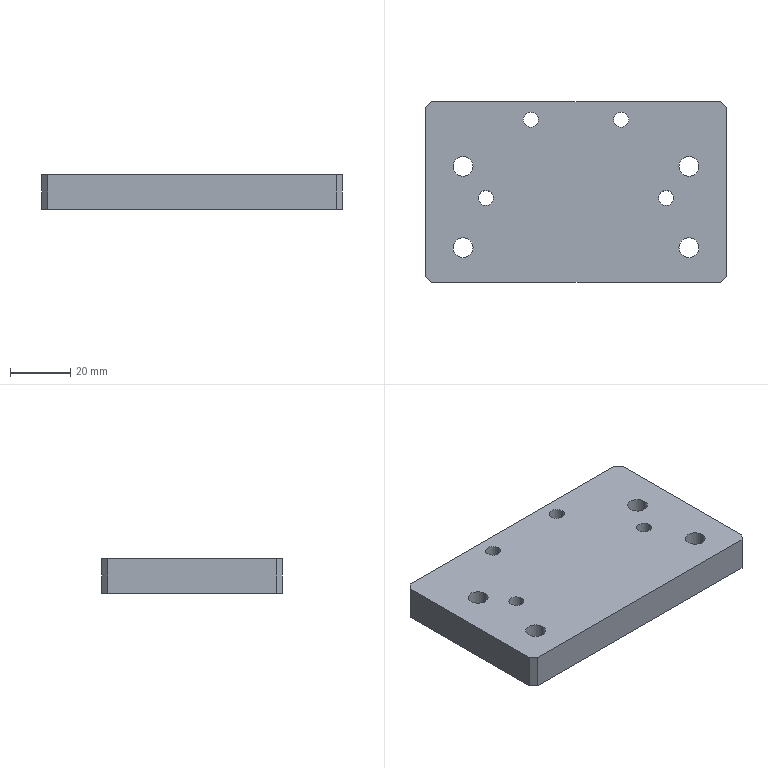Part | STEP file | FBDS-CS-003 | 1 solid | 38 faces | box 100 x 60 x 11.5 mm | volume 64777 mm3 | cylinder 24 | plane 14 | commonest cylinder face diameters 5 x8 6.6 x8 11 x8
STEP:
#1=CARTESIAN_POINT('',(17.5,24.,11.5));
#2=VERTEX_POINT('',#1);
#3=CARTESIAN_POINT('',(12.5,24.,11.5));
#4=VERTEX_POINT('',#3);
#5=CARTESIAN_POINT('',(15.,24.,11.5));
#6=DIRECTION('',(0.,0.,-1.));
#7=DIRECTION('',(-1.,0.,0.));
#8=AXIS2_PLACEMENT_3D('',#5,#6,#7);
#9=CIRCLE('',#8,2.5);
#10=EDGE_CURVE('',#2,#4,#9,.T.);
#11=ORIENTED_EDGE('',*,*,#10,.F.);
#12=CARTESIAN_POINT('',(17.5,24.,0.));
#13=VERTEX_POINT('',#12);
#14=CARTESIAN_POINT('',(17.5,24.,0.));
#15=DIRECTION('',(0.,0.,-1.));
#16=VECTOR('',#15,1000.);
#17=LINE('',#14,#16);
#18=EDGE_CURVE('',#2,#13,#17,.T.);
#19=ORIENTED_EDGE('',*,*,#18,.T.);
#20=CARTESIAN_POINT('',(12.5,24.,0.));
#21=VERTEX_POINT('',#20);
#22=CARTESIAN_POINT('',(15.,24.,0.));
#23=DIRECTION('',(0.,0.,-1.));
#24=DIRECTION('',(-1.,0.,0.));
#25=AXIS2_PLACEMENT_3D('',#22,#23,#24);
#26=CIRCLE('',#25,2.5);
#27=EDGE_CURVE('',#13,#21,#26,.T.);
#28=ORIENTED_EDGE('',*,*,#27,.T.);
#29=CARTESIAN_POINT('',(12.5,24.,0.));
#30=DIRECTION('',(0.,0.,-1.));
#31=VECTOR('',#30,1000.);
#32=LINE('',#29,#31);
#33=EDGE_CURVE('',#4,#21,#32,.T.);
#34=ORIENTED_EDGE('',*,*,#33,.F.);
#35=EDGE_LOOP('',(#11,#19,#28,#34));
#36=FACE_OUTER_BOUND('',#35,.T.);
#37=CARTESIAN_POINT('',(15.,24.,0.));
#38=DIRECTION('',(0.,0.,-1.));
#39=DIRECTION('',(-1.,0.,0.));
#40=AXIS2_PLACEMENT_3D('',#37,#38,#39);
#41=CYLINDRICAL_SURFACE('',#40,2.5);
#42=ADVANCED_FACE('',(#36),#41,.F.);
#43=CARTESIAN_POINT('',(-12.5,24.,11.5));
#44=VERTEX_POINT('',#43);
#45=CARTESIAN_POINT('',(-17.5,24.,11.5));
#46=VERTEX_POINT('',#45);
#47=CARTESIAN_POINT('',(-15.,24.,11.5));
#48=DIRECTION('',(0.,0.,-1.));
#49=DIRECTION('',(-1.,0.,0.));
#50=AXIS2_PLACEMENT_3D('',#47,#48,#49);
#51=CIRCLE('',#50,2.5);
#52=EDGE_CURVE('',#44,#46,#51,.T.);
#53=ORIENTED_EDGE('',*,*,#52,.F.);
#54=CARTESIAN_POINT('',(-12.5,24.,0.));
#55=VERTEX_POINT('',#54);
#56=CARTESIAN_POINT('',(-12.5,24.,0.));
#57=DIRECTION('',(0.,0.,-1.));
#58=VECTOR('',#57,1000.);
#59=LINE('',#56,#58);
#60=EDGE_CURVE('',#44,#55,#59,.T.);
#61=ORIENTED_EDGE('',*,*,#60,.T.);
#62=CARTESIAN_POINT('',(-17.5,24.,0.));
#63=VERTEX_POINT('',#62);
#64=CARTESIAN_POINT('',(-15.,24.,0.));
#65=DIRECTION('',(0.,0.,-1.));
#66=DIRECTION('',(-1.,0.,0.));
#67=AXIS2_PLACEMENT_3D('',#64,#65,#66);
#68=CIRCLE('',#67,2.5);
#69=EDGE_CURVE('',#55,#63,#68,.T.);
#70=ORIENTED_EDGE('',*,*,#69,.T.);
#71=CARTESIAN_POINT('',(-17.5,24.,0.));
#72=DIRECTION('',(0.,0.,-1.));
#73=VECTOR('',#72,1000.);
#74=LINE('',#71,#73);
#75=EDGE_CURVE('',#46,#63,#74,.T.);
#76=ORIENTED_EDGE('',*,*,#75,.F.);
#77=EDGE_LOOP('',(#53,#61,#70,#76));
#78=FACE_OUTER_BOUND('',#77,.T.);
#79=CARTESIAN_POINT('',(-15.,24.,0.));
#80=DIRECTION('',(0.,0.,-1.));
#81=DIRECTION('',(-1.,0.,0.));
#82=AXIS2_PLACEMENT_3D('',#79,#80,#81);
#83=CYLINDRICAL_SURFACE('',#82,2.5);
#84=ADVANCED_FACE('',(#78),#83,.F.);
#85=CARTESIAN_POINT('',(32.5,-2.,11.5));
#86=VERTEX_POINT('',#85);
#87=CARTESIAN_POINT('',(27.5,-2.,11.5));
#88=VERTEX_POINT('',#87);
#89=CARTESIAN_POINT('',(30.,-2.,11.5));
#90=DIRECTION('',(0.,0.,-1.));
#91=DIRECTION('',(-1.,0.,0.));
#92=AXIS2_PLACEMENT_3D('',#89,#90,#91);
#93=CIRCLE('',#92,2.5);
#94=EDGE_CURVE('',#86,#88,#93,.T.);
#95=ORIENTED_EDGE('',*,*,#94,.F.);
#96=CARTESIAN_POINT('',(32.5,-2.,0.));
#97=VERTEX_POINT('',#96);
#98=CARTESIAN_POINT('',(32.5,-2.,0.));
#99=DIRECTION('',(0.,0.,-1.));
#100=VECTOR('',#99,1000.);
#101=LINE('',#98,#100);
#102=EDGE_CURVE('',#86,#97,#101,.T.);
#103=ORIENTED_EDGE('',*,*,#102,.T.);
#104=CARTESIAN_POINT('',(27.5,-2.,0.));
#105=VERTEX_POINT('',#104);
#106=CARTESIAN_POINT('',(30.,-2.,0.));
#107=DIRECTION('',(0.,0.,-1.));
#108=DIRECTION('',(-1.,0.,0.));
#109=AXIS2_PLACEMENT_3D('',#106,#107,#108);
#110=CIRCLE('',#109,2.5);
#111=EDGE_CURVE('',#97,#105,#110,.T.);
#112=ORIENTED_EDGE('',*,*,#111,.T.);
#113=CARTESIAN_POINT('',(27.5,-2.,0.));
#114=DIRECTION('',(0.,0.,-1.));
#115=VECTOR('',#114,1000.);
#116=LINE('',#113,#115);
#117=EDGE_CURVE('',#88,#105,#116,.T.);
#118=ORIENTED_EDGE('',*,*,#117,.F.);
#119=EDGE_LOOP('',(#95,#103,#112,#118));
#120=FACE_OUTER_BOUND('',#119,.T.);
#121=CARTESIAN_POINT('',(30.,-2.,0.));
#122=DIRECTION('',(0.,0.,-1.));
#123=DIRECTION('',(-1.,0.,0.));
#124=AXIS2_PLACEMENT_3D('',#121,#122,#123);
#125=CYLINDRICAL_SURFACE('',#124,2.5);
#126=ADVANCED_FACE('',(#120),#125,.F.);
#127=CARTESIAN_POINT('',(-27.5,-2.,11.5));
#128=VERTEX_POINT('',#127);
#129=CARTESIAN_POINT('',(-32.5,-2.,11.5));
#130=VERTEX_POINT('',#129);
#131=CARTESIAN_POINT('',(-30.,-2.,11.5));
#132=DIRECTION('',(0.,0.,-1.));
#133=DIRECTION('',(-1.,0.,0.));
#134=AXIS2_PLACEMENT_3D('',#131,#132,#133);
#135=CIRCLE('',#134,2.5);
#136=EDGE_CURVE('',#128,#130,#135,.T.);
#137=ORIENTED_EDGE('',*,*,#136,.F.);
#138=CARTESIAN_POINT('',(-27.5,-2.,0.));
#139=VERTEX_POINT('',#138);
#140=CARTESIAN_POINT('',(-27.5,-2.,0.));
#141=DIRECTION('',(0.,0.,-1.));
#142=VECTOR('',#141,1000.);
#143=LINE('',#140,#142);
#144=EDGE_CURVE('',#128,#139,#143,.T.);
#145=ORIENTED_EDGE('',*,*,#144,.T.);
#146=CARTESIAN_POINT('',(-32.5,-2.,0.));
#147=VERTEX_POINT('',#146);
#148=CARTESIAN_POINT('',(-30.,-2.,0.));
#149=DIRECTION('',(0.,0.,-1.));
#150=DIRECTION('',(-1.,0.,0.));
#151=AXIS2_PLACEMENT_3D('',#148,#149,#150);
#152=CIRCLE('',#151,2.5);
#153=EDGE_CURVE('',#139,#147,#152,.T.);
#154=ORIENTED_EDGE('',*,*,#153,.T.);
#155=CARTESIAN_POINT('',(-32.5,-2.,0.));
#156=DIRECTION('',(0.,0.,-1.));
#157=VECTOR('',#156,1000.);
#158=LINE('',#155,#157);
#159=EDGE_CURVE('',#130,#147,#158,.T.);
#160=ORIENTED_EDGE('',*,*,#159,.F.);
#161=EDGE_LOOP('',(#137,#145,#154,#160));
#162=FACE_OUTER_BOUND('',#161,.T.);
#163=CARTESIAN_POINT('',(-30.,-2.,0.));
#164=DIRECTION('',(0.,0.,-1.));
#165=DIRECTION('',(-1.,0.,0.));
#166=AXIS2_PLACEMENT_3D('',#163,#164,#165);
#167=CYLINDRICAL_SURFACE('',#166,2.5);
#168=ADVANCED_FACE('',(#162),#167,.F.);
#169=CARTESIAN_POINT('',(43.,8.5,6.8));
#170=VERTEX_POINT('',#169);
#171=CARTESIAN_POINT('',(32.,8.5,6.8));
#172=VERTEX_POINT('',#171);
#173=CARTESIAN_POINT('',(37.5,8.5,6.8));
#174=DIRECTION('',(0.,0.,-1.));
#175=DIRECTION('',(-1.,0.,0.));
#176=AXIS2_PLACEMENT_3D('',#173,#174,#175);
#177=CIRCLE('',#176,5.5);
#178=EDGE_CURVE('',#170,#172,#177,.T.);
#179=ORIENTED_EDGE('',*,*,#178,.F.);
#180=CARTESIAN_POINT('',(43.,8.5,0.));
#181=VERTEX_POINT('',#180);
#182=CARTESIAN_POINT('',(43.,8.5,0.));
#183=DIRECTION('',(0.,0.,-1.));
#184=VECTOR('',#183,1000.);
#185=LINE('',#182,#184);
#186=EDGE_CURVE('',#170,#181,#185,.T.);
#187=ORIENTED_EDGE('',*,*,#186,.T.);
#188=CARTESIAN_POINT('',(32.,8.5,0.));
#189=VERTEX_POINT('',#188);
#190=CARTESIAN_POINT('',(37.5,8.5,0.));
#191=DIRECTION('',(0.,0.,-1.));
#192=DIRECTION('',(-1.,0.,0.));
#193=AXIS2_PLACEMENT_3D('',#190,#191,#192);
#194=CIRCLE('',#193,5.5);
#195=EDGE_CURVE('',#181,#189,#194,.T.);
#196=ORIENTED_EDGE('',*,*,#195,.T.);
#197=CARTESIAN_POINT('',(32.,8.5,0.));
#198=DIRECTION('',(0.,0.,-1.));
#199=VECTOR('',#198,1000.);
#200=LINE('',#197,#199);
#201=EDGE_CURVE('',#172,#189,#200,.T.);
#202=ORIENTED_EDGE('',*,*,#201,.F.);
#203=EDGE_LOOP('',(#179,#187,#196,#202));
#204=FACE_OUTER_BOUND('',#203,.T.);
#205=CARTESIAN_POINT('',(37.5,8.5,0.));
#206=DIRECTION('',(0.,0.,-1.));
#207=DIRECTION('',(-1.,0.,0.));
#208=AXIS2_PLACEMENT_3D('',#205,#206,#207);
#209=CYLINDRICAL_SURFACE('',#208,5.5);
#210=ADVANCED_FACE('',(#204),#209,.F.);
#211=CARTESIAN_POINT('',(40.8,8.5,11.5));
#212=VERTEX_POINT('',#211);
#213=CARTESIAN_POINT('',(34.2,8.5,11.5));
#214=VERTEX_POINT('',#213);
#215=CARTESIAN_POINT('',(37.5,8.5,11.5));
#216=DIRECTION('',(0.,0.,-1.));
#217=DIRECTION('',(-1.,0.,0.));
#218=AXIS2_PLACEMENT_3D('',#215,#216,#217);
#219=CIRCLE('',#218,3.3);
#220=EDGE_CURVE('',#212,#214,#219,.T.);
#221=ORIENTED_EDGE('',*,*,#220,.F.);
#222=CARTESIAN_POINT('',(40.8,8.5,6.8));
#223=VERTEX_POINT('',#222);
#224=CARTESIAN_POINT('',(40.8,8.5,0.));
#225=DIRECTION('',(0.,0.,-1.));
#226=VECTOR('',#225,1000.);
#227=LINE('',#224,#226);
#228=EDGE_CURVE('',#212,#223,#227,.T.);
#229=ORIENTED_EDGE('',*,*,#228,.T.);
#230=CARTESIAN_POINT('',(34.2,8.5,6.8));
#231=VERTEX_POINT('',#230);
#232=CARTESIAN_POINT('',(37.5,8.5,6.8));
#233=DIRECTION('',(0.,0.,-1.));
#234=DIRECTION('',(-1.,0.,0.));
#235=AXIS2_PLACEMENT_3D('',#232,#233,#234);
#236=CIRCLE('',#235,3.3);
#237=EDGE_CURVE('',#223,#231,#236,.T.);
#238=ORIENTED_EDGE('',*,*,#237,.T.);
#239=CARTESIAN_POINT('',(34.2,8.5,0.));
#240=DIRECTION('',(0.,0.,-1.));
#241=VECTOR('',#240,1000.);
#242=LINE('',#239,#241);
#243=EDGE_CURVE('',#214,#231,#242,.T.);
#244=ORIENTED_EDGE('',*,*,#243,.F.);
#245=EDGE_LOOP('',(#221,#229,#238,#244));
#246=FACE_OUTER_BOUND('',#245,.T.);
#247=CARTESIAN_POINT('',(37.5,8.5,0.));
#248=DIRECTION('',(0.,0.,-1.));
#249=DIRECTION('',(-1.,0.,0.));
#250=AXIS2_PLACEMENT_3D('',#247,#248,#249);
#251=CYLINDRICAL_SURFACE('',#250,3.3);
#252=ADVANCED_FACE('',(#246),#251,.F.);
#253=CARTESIAN_POINT('',(-32.,8.5,6.8));
#254=VERTEX_POINT('',#253);
#255=CARTESIAN_POINT('',(-43.,8.5,6.8));
#256=VERTEX_POINT('',#255);
#257=CARTESIAN_POINT('',(-37.5,8.5,6.8));
#258=DIRECTION('',(0.,0.,-1.));
#259=DIRECTION('',(-1.,0.,0.));
#260=AXIS2_PLACEMENT_3D('',#257,#258,#259);
#261=CIRCLE('',#260,5.5);
#262=EDGE_CURVE('',#254,#256,#261,.T.);
#263=ORIENTED_EDGE('',*,*,#262,.F.);
#264=CARTESIAN_POINT('',(-32.,8.5,0.));
#265=VERTEX_POINT('',#264);
#266=CARTESIAN_POINT('',(-32.,8.5,0.));
#267=DIRECTION('',(0.,0.,-1.));
#268=VECTOR('',#267,1000.);
#269=LINE('',#266,#268);
#270=EDGE_CURVE('',#254,#265,#269,.T.);
#271=ORIENTED_EDGE('',*,*,#270,.T.);
#272=CARTESIAN_POINT('',(-43.,8.5,0.));
#273=VERTEX_POINT('',#272);
#274=CARTESIAN_POINT('',(-37.5,8.5,0.));
#275=DIRECTION('',(0.,0.,-1.));
#276=DIRECTION('',(-1.,0.,0.));
#277=AXIS2_PLACEMENT_3D('',#274,#275,#276);
#278=CIRCLE('',#277,5.5);
#279=EDGE_CURVE('',#265,#273,#278,.T.);
#280=ORIENTED_EDGE('',*,*,#279,.T.);
#281=CARTESIAN_POINT('',(-43.,8.5,0.));
#282=DIRECTION('',(0.,0.,-1.));
#283=VECTOR('',#282,1000.);
#284=LINE('',#281,#283);
#285=EDGE_CURVE('',#256,#273,#284,.T.);
#286=ORIENTED_EDGE('',*,*,#285,.F.);
#287=EDGE_LOOP('',(#263,#271,#280,#286));
#288=FACE_OUTER_BOUND('',#287,.T.);
#289=CARTESIAN_POINT('',(-37.5,8.5,0.));
#290=DIRECTION('',(0.,0.,-1.));
#291=DIRECTION('',(-1.,0.,0.));
#292=AXIS2_PLACEMENT_3D('',#289,#290,#291);
#293=CYLINDRICAL_SURFACE('',#292,5.5);
#294=ADVANCED_FACE('',(#288),#293,.F.);
#295=CARTESIAN_POINT('',(-34.2,8.5,11.5));
#296=VERTEX_POINT('',#295);
#297=CARTESIAN_POINT('',(-40.8,8.5,11.5));
#298=VERTEX_POINT('',#297);
#299=CARTESIAN_POINT('',(-37.5,8.5,11.5));
#300=DIRECTION('',(0.,0.,-1.));
#301=DIRECTION('',(-1.,0.,0.));
#302=AXIS2_PLACEMENT_3D('',#299,#300,#301);
#303=CIRCLE('',#302,3.3);
#304=EDGE_CURVE('',#296,#298,#303,.T.);
#305=ORIENTED_EDGE('',*,*,#304,.F.);
#306=CARTESIAN_POINT('',(-34.2,8.5,6.8));
#307=VERTEX_POINT('',#306);
#308=CARTESIAN_POINT('',(-34.2,8.5,0.));
#309=DIRECTION('',(0.,0.,-1.));
#310=VECTOR('',#309,1000.);
#311=LINE('',#308,#310);
#312=EDGE_CURVE('',#296,#307,#311,.T.);
#313=ORIENTED_EDGE('',*,*,#312,.T.);
#314=CARTESIAN_POINT('',(-40.8,8.5,6.8));
#315=VERTEX_POINT('',#314);
#316=CARTESIAN_POINT('',(-37.5,8.5,6.8));
#317=DIRECTION('',(0.,0.,-1.));
#318=DIRECTION('',(-1.,0.,0.));
#319=AXIS2_PLACEMENT_3D('',#316,#317,#318);
#320=CIRCLE('',#319,3.3);
#321=EDGE_CURVE('',#307,#315,#320,.T.);
#322=ORIENTED_EDGE('',*,*,#321,.T.);
#323=CARTESIAN_POINT('',(-40.8,8.5,0.));
#324=DIRECTION('',(0.,0.,-1.));
#325=VECTOR('',#324,1000.);
#326=LINE('',#323,#325);
#327=EDGE_CURVE('',#298,#315,#326,.T.);
#328=ORIENTED_EDGE('',*,*,#327,.F.);
#329=EDGE_LOOP('',(#305,#313,#322,#328));
#330=FACE_OUTER_BOUND('',#329,.T.);
#331=CARTESIAN_POINT('',(-37.5,8.5,0.));
#332=DIRECTION('',(0.,0.,-1.));
#333=DIRECTION('',(-1.,0.,0.));
#334=AXIS2_PLACEMENT_3D('',#331,#332,#333);
#335=CYLINDRICAL_SURFACE('',#334,3.3);
#336=ADVANCED_FACE('',(#330),#335,.F.);
#337=CARTESIAN_POINT('',(-32.,-18.5,6.8));
#338=VERTEX_POINT('',#337);
#339=CARTESIAN_POINT('',(-43.,-18.5,6.8));
#340=VERTEX_POINT('',#339);
#341=CARTESIAN_POINT('',(-37.5,-18.5,6.8));
#342=DIRECTION('',(0.,0.,-1.));
#343=DIRECTION('',(-1.,0.,0.));
#344=AXIS2_PLACEMENT_3D('',#341,#342,#343);
#345=CIRCLE('',#344,5.5);
#346=EDGE_CURVE('',#338,#340,#345,.T.);
#347=ORIENTED_EDGE('',*,*,#346,.F.);
#348=CARTESIAN_POINT('',(-32.,-18.5,0.));
#349=VERTEX_POINT('',#348);
#350=CARTESIAN_POINT('',(-32.,-18.5,0.));
#351=DIRECTION('',(0.,0.,-1.));
#352=VECTOR('',#351,1000.);
#353=LINE('',#350,#352);
#354=EDGE_CURVE('',#338,#349,#353,.T.);
#355=ORIENTED_EDGE('',*,*,#354,.T.);
#356=CARTESIAN_POINT('',(-43.,-18.5,0.));
#357=VERTEX_POINT('',#356);
#358=CARTESIAN_POINT('',(-37.5,-18.5,0.));
#359=DIRECTION('',(0.,0.,-1.));
#360=DIRECTION('',(-1.,0.,0.));
#361=AXIS2_PLACEMENT_3D('',#358,#359,#360);
#362=CIRCLE('',#361,5.5);
#363=EDGE_CURVE('',#349,#357,#362,.T.);
#364=ORIENTED_EDGE('',*,*,#363,.T.);
#365=CARTESIAN_POINT('',(-43.,-18.5,0.));
#366=DIRECTION('',(0.,0.,-1.));
#367=VECTOR('',#366,1000.);
#368=LINE('',#365,#367);
#369=EDGE_CURVE('',#340,#357,#368,.T.);
#370=ORIENTED_EDGE('',*,*,#369,.F.);
#371=EDGE_LOOP('',(#347,#355,#364,#370));
#372=FACE_OUTER_BOUND('',#371,.T.);
#373=CARTESIAN_POINT('',(-37.5,-18.5,0.));
#374=DIRECTION('',(0.,0.,-1.));
#375=DIRECTION('',(-1.,0.,0.));
#376=AXIS2_PLACEMENT_3D('',#373,#374,#375);
#377=CYLINDRICAL_SURFACE('',#376,5.5);
#378=ADVANCED_FACE('',(#372),#377,.F.);
#379=CARTESIAN_POINT('',(-34.2,-18.5,11.5));
#380=VERTEX_POINT('',#379);
#381=CARTESIAN_POINT('',(-40.8,-18.5,11.5));
#382=VERTEX_POINT('',#381);
#383=CARTESIAN_POINT('',(-37.5,-18.5,11.5));
#384=DIRECTION('',(0.,0.,-1.));
#385=DIRECTION('',(-1.,0.,0.));
#386=AXIS2_PLACEMENT_3D('',#383,#384,#385);
#387=CIRCLE('',#386,3.3);
#388=EDGE_CURVE('',#380,#382,#387,.T.);
#389=ORIENTED_EDGE('',*,*,#388,.F.);
#390=CARTESIAN_POINT('',(-34.2,-18.5,6.8));
#391=VERTEX_POINT('',#390);
#392=CARTESIAN_POINT('',(-34.2,-18.5,0.));
#393=DIRECTION('',(0.,0.,-1.));
#394=VECTOR('',#393,1000.);
#395=LINE('',#392,#394);
#396=EDGE_CURVE('',#380,#391,#395,.T.);
#397=ORIENTED_EDGE('',*,*,#396,.T.);
#398=CARTESIAN_POINT('',(-40.8,-18.5,6.8));
#399=VERTEX_POINT('',#398);
#400=CARTESIAN_POINT('',(-37.5,-18.5,6.8));
#401=DIRECTION('',(0.,0.,-1.));
#402=DIRECTION('',(-1.,0.,0.));
#403=AXIS2_PLACEMENT_3D('',#400,#401,#402);
#404=CIRCLE('',#403,3.3);
#405=EDGE_CURVE('',#391,#399,#404,.T.);
#406=ORIENTED_EDGE('',*,*,#405,.T.);
#407=CARTESIAN_POINT('',(-40.8,-18.5,0.));
#408=DIRECTION('',(0.,0.,-1.));
#409=VECTOR('',#408,1000.);
#410=LINE('',#407,#409);
#411=EDGE_CURVE('',#382,#399,#410,.T.);
#412=ORIENTED_EDGE('',*,*,#411,.F.);
#413=EDGE_LOOP('',(#389,#397,#406,#412));
#414=FACE_OUTER_BOUND('',#413,.T.);
#415=CARTESIAN_POINT('',(-37.5,-18.5,0.));
#416=DIRECTION('',(0.,0.,-1.));
#417=DIRECTION('',(-1.,0.,0.));
#418=AXIS2_PLACEMENT_3D('',#415,#416,#417);
#419=CYLINDRICAL_SURFACE('',#418,3.3);
#420=ADVANCED_FACE('',(#414),#419,.F.);
#421=CARTESIAN_POINT('',(43.,-18.5,6.8));
#422=VERTEX_POINT('',#421);
#423=CARTESIAN_POINT('',(32.,-18.5,6.8));
#424=VERTEX_POINT('',#423);
#425=CARTESIAN_POINT('',(37.5,-18.5,6.8));
#426=DIRECTION('',(0.,0.,-1.));
#427=DIRECTION('',(-1.,0.,0.));
#428=AXIS2_PLACEMENT_3D('',#425,#426,#427);
#429=CIRCLE('',#428,5.5);
#430=EDGE_CURVE('',#422,#424,#429,.T.);
#431=ORIENTED_EDGE('',*,*,#430,.F.);
#432=CARTESIAN_POINT('',(43.,-18.5,0.));
#433=VERTEX_POINT('',#432);
#434=CARTESIAN_POINT('',(43.,-18.5,0.));
#435=DIRECTION('',(0.,0.,-1.));
#436=VECTOR('',#435,1000.);
#437=LINE('',#434,#436);
#438=EDGE_CURVE('',#422,#433,#437,.T.);
#439=ORIENTED_EDGE('',*,*,#438,.T.);
#440=CARTESIAN_POINT('',(32.,-18.5,0.));
#441=VERTEX_POINT('',#440);
#442=CARTESIAN_POINT('',(37.5,-18.5,0.));
#443=DIRECTION('',(0.,0.,-1.));
#444=DIRECTION('',(-1.,0.,0.));
#445=AXIS2_PLACEMENT_3D('',#442,#443,#444);
#446=CIRCLE('',#445,5.5);
#447=EDGE_CURVE('',#433,#441,#446,.T.);
#448=ORIENTED_EDGE('',*,*,#447,.T.);
#449=CARTESIAN_POINT('',(32.,-18.5,0.));
#450=DIRECTION('',(0.,0.,-1.));
#451=VECTOR('',#450,1000.);
#452=LINE('',#449,#451);
#453=EDGE_CURVE('',#424,#441,#452,.T.);
#454=ORIENTED_EDGE('',*,*,#453,.F.);
#455=EDGE_LOOP('',(#431,#439,#448,#454));
#456=FACE_OUTER_BOUND('',#455,.T.);
#457=CARTESIAN_POINT('',(37.5,-18.5,0.));
#458=DIRECTION('',(0.,0.,-1.));
#459=DIRECTION('',(-1.,0.,0.));
#460=AXIS2_PLACEMENT_3D('',#457,#458,#459);
#461=CYLINDRICAL_SURFACE('',#460,5.5);
#462=ADVANCED_FACE('',(#456),#461,.F.);
#463=CARTESIAN_POINT('',(40.8,-18.5,11.5));
#464=VERTEX_POINT('',#463);
#465=CARTESIAN_POINT('',(34.2,-18.5,11.5));
#466=VERTEX_POINT('',#465);
#467=CARTESIAN_POINT('',(37.5,-18.5,11.5));
#468=DIRECTION('',(0.,0.,-1.));
#469=DIRECTION('',(-1.,0.,0.));
#470=AXIS2_PLACEMENT_3D('',#467,#468,#469);
#471=CIRCLE('',#470,3.3);
#472=EDGE_CURVE('',#464,#466,#471,.T.);
#473=ORIENTED_EDGE('',*,*,#472,.F.);
#474=CARTESIAN_POINT('',(40.8,-18.5,6.8));
#475=VERTEX_POINT('',#474);
#476=CARTESIAN_POINT('',(40.8,-18.5,0.));
#477=DIRECTION('',(0.,0.,-1.));
#478=VECTOR('',#477,1000.);
#479=LINE('',#476,#478);
#480=EDGE_CURVE('',#464,#475,#479,.T.);
#481=ORIENTED_EDGE('',*,*,#480,.T.);
#482=CARTESIAN_POINT('',(34.2,-18.5,6.8));
#483=VERTEX_POINT('',#482);
#484=CARTESIAN_POINT('',(37.5,-18.5,6.8));
#485=DIRECTION('',(0.,0.,-1.));
#486=DIRECTION('',(-1.,0.,0.));
#487=AXIS2_PLACEMENT_3D('',#484,#485,#486);
#488=CIRCLE('',#487,3.3);
#489=EDGE_CURVE('',#475,#483,#488,.T.);
#490=ORIENTED_EDGE('',*,*,#489,.T.);
#491=CARTESIAN_POINT('',(34.2,-18.5,0.));
#492=DIRECTION('',(0.,0.,-1.));
#493=VECTOR('',#492,1000.);
#494=LINE('',#491,#493);
#495=EDGE_CURVE('',#466,#483,#494,.T.);
#496=ORIENTED_EDGE('',*,*,#495,.F.);
#497=EDGE_LOOP('',(#473,#481,#490,#496));
#498=FACE_OUTER_BOUND('',#497,.T.);
#499=CARTESIAN_POINT('',(37.5,-18.5,0.));
#500=DIRECTION('',(0.,0.,-1.));
#501=DIRECTION('',(-1.,0.,0.));
#502=AXIS2_PLACEMENT_3D('',#499,#500,#501);
#503=CYLINDRICAL_SURFACE('',#502,3.3);
#504=ADVANCED_FACE('',(#498),#503,.F.);
#505=CARTESIAN_POINT('',(50.,-28.,11.5));
#506=VERTEX_POINT('',#505);
#507=CARTESIAN_POINT('',(50.,28.,11.5));
#508=VERTEX_POINT('',#507);
#509=CARTESIAN_POINT('',(50.,-30.,11.5));
#510=DIRECTION('',(0.,1.,0.));
#511=VECTOR('',#510,1000.);
#512=LINE('',#509,#511);
#513=EDGE_CURVE('',#506,#508,#512,.T.);
#514=ORIENTED_EDGE('',*,*,#513,.F.);
#515=CARTESIAN_POINT('',(50.,-28.,0.));
#516=VERTEX_POINT('',#515);
#517=CARTESIAN_POINT('',(50.,-28.,11.5));
#518=DIRECTION('',(0.,0.,-1.));
#519=VECTOR('',#518,1000.);
#520=LINE('',#517,#519);
#521=EDGE_CURVE('',#506,#516,#520,.T.);
#522=ORIENTED_EDGE('',*,*,#521,.T.);
#523=CARTESIAN_POINT('',(50.,28.,0.));
#524=VERTEX_POINT('',#523);
#525=CARTESIAN_POINT('',(50.,-30.,0.));
#526=DIRECTION('',(0.,1.,0.));
#527=VECTOR('',#526,1000.);
#528=LINE('',#525,#527);
#529=EDGE_CURVE('',#516,#524,#528,.T.);
#530=ORIENTED_EDGE('',*,*,#529,.T.);
#531=CARTESIAN_POINT('',(50.,28.,11.5));
#532=DIRECTION('',(0.,0.,1.));
#533=VECTOR('',#532,1000.);
#534=LINE('',#531,#533);
#535=EDGE_CURVE('',#524,#508,#534,.T.);
#536=ORIENTED_EDGE('',*,*,#535,.T.);
#537=EDGE_LOOP('',(#514,#522,#530,#536));
#538=FACE_OUTER_BOUND('',#537,.T.);
#539=CARTESIAN_POINT('',(50.,-30.,11.5));
#540=DIRECTION('',(-1.,0.,0.));
#541=DIRECTION('',(0.,0.,1.));
#542=AXIS2_PLACEMENT_3D('',#539,#540,#541);
#543=PLANE('',#542);
#544=ADVANCED_FACE('',(#538),#543,.F.);
#545=CARTESIAN_POINT('',(48.,30.,0.));
#546=VERTEX_POINT('',#545);
#547=CARTESIAN_POINT('',(-48.,30.,0.));
#548=VERTEX_POINT('',#547);
#549=CARTESIAN_POINT('',(-50.,30.,0.));
#550=DIRECTION('',(-1.,0.,0.));
#551=VECTOR('',#550,1000.);
#552=LINE('',#549,#551);
#553=EDGE_CURVE('',#546,#548,#552,.T.);
#554=ORIENTED_EDGE('',*,*,#553,.T.);
#555=CARTESIAN_POINT('',(-48.,30.,11.5));
#556=VERTEX_POINT('',#555);
#557=CARTESIAN_POINT('',(-48.,30.,11.5));
#558=DIRECTION('',(0.,0.,1.));
#559=VECTOR('',#558,1000.);
#560=LINE('',#557,#559);
#561=EDGE_CURVE('',#548,#556,#560,.T.);
#562=ORIENTED_EDGE('',*,*,#561,.T.);
#563=CARTESIAN_POINT('',(48.,30.,11.5));
#564=VERTEX_POINT('',#563);
#565=CARTESIAN_POINT('',(-50.,30.,11.5));
#566=DIRECTION('',(-1.,0.,0.));
#567=VECTOR('',#566,1000.);
#568=LINE('',#565,#567);
#569=EDGE_CURVE('',#564,#556,#568,.T.);
#570=ORIENTED_EDGE('',*,*,#569,.F.);
#571=CARTESIAN_POINT('',(48.,30.,11.5));
#572=DIRECTION('',(0.,0.,-1.));
#573=VECTOR('',#572,1000.);
#574=LINE('',#571,#573);
#575=EDGE_CURVE('',#564,#546,#574,.T.);
#576=ORIENTED_EDGE('',*,*,#575,.T.);
#577=EDGE_LOOP('',(#554,#562,#570,#576));
#578=FACE_OUTER_BOUND('',#577,.T.);
#579=CARTESIAN_POINT('',(-50.,30.,11.5));
#580=DIRECTION('',(0.,-1.,0.));
#581=DIRECTION('',(0.,0.,-1.));
#582=AXIS2_PLACEMENT_3D('',#579,#580,#581);
#583=PLANE('',#582);
#584=ADVANCED_FACE('',(#578),#583,.F.);
#585=CARTESIAN_POINT('',(-50.,28.,0.));
#586=VERTEX_POINT('',#585);
#587=CARTESIAN_POINT('',(-50.,-28.,0.));
#588=VERTEX_POINT('',#587);
#589=CARTESIAN_POINT('',(-50.,-30.,0.));
#590=DIRECTION('',(0.,-1.,0.));
#591=VECTOR('',#590,1000.);
#592=LINE('',#589,#591);
#593=EDGE_CURVE('',#586,#588,#592,.T.);
#594=ORIENTED_EDGE('',*,*,#593,.T.);
#595=CARTESIAN_POINT('',(-50.,-28.,11.5));
#596=VERTEX_POINT('',#595);
#597=CARTESIAN_POINT('',(-50.,-28.,11.5));
#598=DIRECTION('',(0.,0.,1.));
#599=VECTOR('',#598,1000.);
#600=LINE('',#597,#599);
#601=EDGE_CURVE('',#588,#596,#600,.T.);
#602=ORIENTED_EDGE('',*,*,#601,.T.);
#603=CARTESIAN_POINT('',(-50.,28.,11.5));
#604=VERTEX_POINT('',#603);
#605=CARTESIAN_POINT('',(-50.,-30.,11.5));
#606=DIRECTION('',(0.,-1.,0.));
#607=VECTOR('',#606,1000.);
#608=LINE('',#605,#607);
#609=EDGE_CURVE('',#604,#596,#608,.T.);
#610=ORIENTED_EDGE('',*,*,#609,.F.);
#611=CARTESIAN_POINT('',(-50.,28.,11.5));
#612=DIRECTION('',(0.,0.,-1.));
#613=VECTOR('',#612,1000.);
#614=LINE('',#611,#613);
#615=EDGE_CURVE('',#604,#586,#614,.T.);
#616=ORIENTED_EDGE('',*,*,#615,.T.);
#617=EDGE_LOOP('',(#594,#602,#610,#616));
#618=FACE_OUTER_BOUND('',#617,.T.);
#619=CARTESIAN_POINT('',(-50.,-30.,11.5));
#620=DIRECTION('',(1.,0.,0.));
#621=DIRECTION('',(0.,0.,-1.));
#622=AXIS2_PLACEMENT_3D('',#619,#620,#621);
#623=PLANE('',#622);
#624=ADVANCED_FACE('',(#618),#623,.F.);
#625=CARTESIAN_POINT('',(-48.,-30.,11.5));
#626=VERTEX_POINT('',#625);
#627=CARTESIAN_POINT('',(48.,-30.,11.5));
#628=VERTEX_POINT('',#627);
#629=CARTESIAN_POINT('',(-50.,-30.,11.5));
#630=DIRECTION('',(1.,0.,0.));
#631=VECTOR('',#630,1000.);
#632=LINE('',#629,#631);
#633=EDGE_CURVE('',#626,#628,#632,.T.);
#634=ORIENTED_EDGE('',*,*,#633,.F.);
#635=CARTESIAN_POINT('',(-48.,-30.,0.));
#636=VERTEX_POINT('',#635);
#637=CARTESIAN_POINT('',(-48.,-30.,11.5));
#638=DIRECTION('',(0.,0.,-1.));
#639=VECTOR('',#638,1000.);
#640=LINE('',#637,#639);
#641=EDGE_CURVE('',#626,#636,#640,.T.);
#642=ORIENTED_EDGE('',*,*,#641,.T.);
#643=CARTESIAN_POINT('',(48.,-30.,0.));
#644=VERTEX_POINT('',#643);
#645=CARTESIAN_POINT('',(-50.,-30.,0.));
#646=DIRECTION('',(1.,0.,0.));
#647=VECTOR('',#646,1000.);
#648=LINE('',#645,#647);
#649=EDGE_CURVE('',#636,#644,#648,.T.);
#650=ORIENTED_EDGE('',*,*,#649,.T.);
#651=CARTESIAN_POINT('',(48.,-30.,11.5));
#652=DIRECTION('',(0.,0.,1.));
#653=VECTOR('',#652,1000.);
#654=LINE('',#651,#653);
#655=EDGE_CURVE('',#644,#628,#654,.T.);
#656=ORIENTED_EDGE('',*,*,#655,.T.);
#657=EDGE_LOOP('',(#634,#642,#650,#656));
#658=FACE_OUTER_BOUND('',#657,.T.);
#659=CARTESIAN_POINT('',(-50.,-30.,11.5));
#660=DIRECTION('',(0.,1.,0.));
#661=DIRECTION('',(0.,0.,1.));
#662=AXIS2_PLACEMENT_3D('',#659,#660,#661);
#663=PLANE('',#662);
#664=ADVANCED_FACE('',(#658),#663,.F.);
#665=CARTESIAN_POINT('',(15.,24.,11.5));
#666=DIRECTION('',(0.,0.,-1.));
#667=DIRECTION('',(-1.,0.,0.));
#668=AXIS2_PLACEMENT_3D('',#665,#666,#667);
#669=CIRCLE('',#668,2.5);
#670=EDGE_CURVE('',#4,#2,#669,.T.);
#671=ORIENTED_EDGE('',*,*,#670,.T.);
#672=ORIENTED_EDGE('',*,*,#10,.T.);
#673=EDGE_LOOP('',(#671,#672));
#674=FACE_BOUND('',#673,.T.);
#675=CARTESIAN_POINT('',(-15.,24.,11.5));
#676=DIRECTION('',(0.,0.,-1.));
#677=DIRECTION('',(-1.,0.,0.));
#678=AXIS2_PLACEMENT_3D('',#675,#676,#677);
#679=CIRCLE('',#678,2.5);
#680=EDGE_CURVE('',#46,#44,#679,.T.);
#681=ORIENTED_EDGE('',*,*,#680,.T.);
#682=ORIENTED_EDGE('',*,*,#52,.T.);
#683=EDGE_LOOP('',(#681,#682));
#684=FACE_BOUND('',#683,.T.);
#685=CARTESIAN_POINT('',(30.,-2.,11.5));
#686=DIRECTION('',(0.,0.,-1.));
#687=DIRECTION('',(-1.,0.,0.));
#688=AXIS2_PLACEMENT_3D('',#685,#686,#687);
#689=CIRCLE('',#688,2.5);
#690=EDGE_CURVE('',#88,#86,#689,.T.);
#691=ORIENTED_EDGE('',*,*,#690,.T.);
#692=ORIENTED_EDGE('',*,*,#94,.T.);
#693=EDGE_LOOP('',(#691,#692));
#694=FACE_BOUND('',#693,.T.);
#695=CARTESIAN_POINT('',(-30.,-2.,11.5));
#696=DIRECTION('',(0.,0.,-1.));
#697=DIRECTION('',(-1.,0.,0.));
#698=AXIS2_PLACEMENT_3D('',#695,#696,#697);
#699=CIRCLE('',#698,2.5);
#700=EDGE_CURVE('',#130,#128,#699,.T.);
#701=ORIENTED_EDGE('',*,*,#700,.T.);
#702=ORIENTED_EDGE('',*,*,#136,.T.);
#703=EDGE_LOOP('',(#701,#702));
#704=FACE_BOUND('',#703,.T.);
#705=CARTESIAN_POINT('',(37.5,8.5,11.5));
#706=DIRECTION('',(0.,0.,-1.));
#707=DIRECTION('',(-1.,0.,0.));
#708=AXIS2_PLACEMENT_3D('',#705,#706,#707);
#709=CIRCLE('',#708,3.3);
#710=EDGE_CURVE('',#214,#212,#709,.T.);
#711=ORIENTED_EDGE('',*,*,#710,.T.);
#712=ORIENTED_EDGE('',*,*,#220,.T.);
#713=EDGE_LOOP('',(#711,#712));
#714=FACE_BOUND('',#713,.T.);
#715=CARTESIAN_POINT('',(-37.5,8.5,11.5));
#716=DIRECTION('',(0.,0.,-1.));
#717=DIRECTION('',(-1.,0.,0.));
#718=AXIS2_PLACEMENT_3D('',#715,#716,#717);
#719=CIRCLE('',#718,3.3);
#720=EDGE_CURVE('',#298,#296,#719,.T.);
#721=ORIENTED_EDGE('',*,*,#720,.T.);
#722=ORIENTED_EDGE('',*,*,#304,.T.);
#723=EDGE_LOOP('',(#721,#722));
#724=FACE_BOUND('',#723,.T.);
#725=CARTESIAN_POINT('',(-37.5,-18.5,11.5));
#726=DIRECTION('',(0.,0.,-1.));
#727=DIRECTION('',(-1.,0.,0.));
#728=AXIS2_PLACEMENT_3D('',#725,#726,#727);
#729=CIRCLE('',#728,3.3);
#730=EDGE_CURVE('',#382,#380,#729,.T.);
#731=ORIENTED_EDGE('',*,*,#730,.T.);
#732=ORIENTED_EDGE('',*,*,#388,.T.);
#733=EDGE_LOOP('',(#731,#732));
#734=FACE_BOUND('',#733,.T.);
#735=CARTESIAN_POINT('',(37.5,-18.5,11.5));
#736=DIRECTION('',(0.,0.,-1.));
#737=DIRECTION('',(-1.,0.,0.));
#738=AXIS2_PLACEMENT_3D('',#735,#736,#737);
#739=CIRCLE('',#738,3.3);
#740=EDGE_CURVE('',#466,#464,#739,.T.);
#741=ORIENTED_EDGE('',*,*,#740,.T.);
#742=ORIENTED_EDGE('',*,*,#472,.T.);
#743=EDGE_LOOP('',(#741,#742));
#744=FACE_BOUND('',#743,.T.);
#745=ORIENTED_EDGE('',*,*,#609,.T.);
#746=CARTESIAN_POINT('',(-48.,-30.,11.5));
#747=DIRECTION('',(0.7071,-0.7071,0.));
#748=VECTOR('',#747,1000.);
#749=LINE('',#746,#748);
#750=EDGE_CURVE('',#596,#626,#749,.T.);
#751=ORIENTED_EDGE('',*,*,#750,.T.);
#752=ORIENTED_EDGE('',*,*,#633,.T.);
#753=CARTESIAN_POINT('',(50.,-28.,11.5));
#754=DIRECTION('',(0.7071,0.7071,0.));
#755=VECTOR('',#754,1000.);
#756=LINE('',#753,#755);
#757=EDGE_CURVE('',#628,#506,#756,.T.);
#758=ORIENTED_EDGE('',*,*,#757,.T.);
#759=ORIENTED_EDGE('',*,*,#513,.T.);
#760=CARTESIAN_POINT('',(48.,30.,11.5));
#761=DIRECTION('',(-0.7071,0.7071,0.));
#762=VECTOR('',#761,1000.);
#763=LINE('',#760,#762);
#764=EDGE_CURVE('',#508,#564,#763,.T.);
#765=ORIENTED_EDGE('',*,*,#764,.T.);
#766=ORIENTED_EDGE('',*,*,#569,.T.);
#767=CARTESIAN_POINT('',(-50.,28.,11.5));
#768=DIRECTION('',(-0.7071,-0.7071,0.));
#769=VECTOR('',#768,1000.);
#770=LINE('',#767,#769);
#771=EDGE_CURVE('',#556,#604,#770,.T.);
#772=ORIENTED_EDGE('',*,*,#771,.T.);
#773=EDGE_LOOP('',(#745,#751,#752,#758,#759,#765,#766,#772));
#774=FACE_OUTER_BOUND('',#773,.T.);
#775=CARTESIAN_POINT('',(0.,0.,11.5));
#776=DIRECTION('',(0.,0.,-1.));
#777=DIRECTION('',(-1.,0.,0.));
#778=AXIS2_PLACEMENT_3D('',#775,#776,#777);
#779=PLANE('',#778);
#780=ADVANCED_FACE('',(#674,#684,#694,#704,#714,#724,#734,#744,#774),#779,.F.);
#781=CARTESIAN_POINT('',(15.,24.,0.));
#782=DIRECTION('',(0.,0.,-1.));
#783=DIRECTION('',(-1.,0.,0.));
#784=AXIS2_PLACEMENT_3D('',#781,#782,#783);
#785=CIRCLE('',#784,2.5);
#786=EDGE_CURVE('',#21,#13,#785,.T.);
#787=ORIENTED_EDGE('',*,*,#786,.F.);
#788=ORIENTED_EDGE('',*,*,#27,.F.);
#789=EDGE_LOOP('',(#787,#788));
#790=FACE_BOUND('',#789,.T.);
#791=CARTESIAN_POINT('',(-15.,24.,0.));
#792=DIRECTION('',(0.,0.,-1.));
#793=DIRECTION('',(-1.,0.,0.));
#794=AXIS2_PLACEMENT_3D('',#791,#792,#793);
#795=CIRCLE('',#794,2.5);
#796=EDGE_CURVE('',#63,#55,#795,.T.);
#797=ORIENTED_EDGE('',*,*,#796,.F.);
#798=ORIENTED_EDGE('',*,*,#69,.F.);
#799=EDGE_LOOP('',(#797,#798));
#800=FACE_BOUND('',#799,.T.);
#801=CARTESIAN_POINT('',(30.,-2.,0.));
#802=DIRECTION('',(0.,0.,-1.));
#803=DIRECTION('',(-1.,0.,0.));
#804=AXIS2_PLACEMENT_3D('',#801,#802,#803);
#805=CIRCLE('',#804,2.5);
#806=EDGE_CURVE('',#105,#97,#805,.T.);
#807=ORIENTED_EDGE('',*,*,#806,.F.);
#808=ORIENTED_EDGE('',*,*,#111,.F.);
#809=EDGE_LOOP('',(#807,#808));
#810=FACE_BOUND('',#809,.T.);
#811=CARTESIAN_POINT('',(-30.,-2.,0.));
#812=DIRECTION('',(0.,0.,-1.));
#813=DIRECTION('',(-1.,0.,0.));
#814=AXIS2_PLACEMENT_3D('',#811,#812,#813);
#815=CIRCLE('',#814,2.5);
#816=EDGE_CURVE('',#147,#139,#815,.T.);
#817=ORIENTED_EDGE('',*,*,#816,.F.);
#818=ORIENTED_EDGE('',*,*,#153,.F.);
#819=EDGE_LOOP('',(#817,#818));
#820=FACE_BOUND('',#819,.T.);
#821=CARTESIAN_POINT('',(37.5,8.5,0.));
#822=DIRECTION('',(0.,0.,-1.));
#823=DIRECTION('',(-1.,0.,0.));
#824=AXIS2_PLACEMENT_3D('',#821,#822,#823);
#825=CIRCLE('',#824,5.5);
#826=EDGE_CURVE('',#189,#181,#825,.T.);
#827=ORIENTED_EDGE('',*,*,#826,.F.);
#828=ORIENTED_EDGE('',*,*,#195,.F.);
#829=EDGE_LOOP('',(#827,#828));
#830=FACE_BOUND('',#829,.T.);
#831=CARTESIAN_POINT('',(-37.5,8.5,0.));
#832=DIRECTION('',(0.,0.,-1.));
#833=DIRECTION('',(-1.,0.,0.));
#834=AXIS2_PLACEMENT_3D('',#831,#832,#833);
#835=CIRCLE('',#834,5.5);
#836=EDGE_CURVE('',#273,#265,#835,.T.);
#837=ORIENTED_EDGE('',*,*,#836,.F.);
#838=ORIENTED_EDGE('',*,*,#279,.F.);
#839=EDGE_LOOP('',(#837,#838));
#840=FACE_BOUND('',#839,.T.);
#841=CARTESIAN_POINT('',(-37.5,-18.5,0.));
#842=DIRECTION('',(0.,0.,-1.));
#843=DIRECTION('',(-1.,0.,0.));
#844=AXIS2_PLACEMENT_3D('',#841,#842,#843);
#845=CIRCLE('',#844,5.5);
#846=EDGE_CURVE('',#357,#349,#845,.T.);
#847=ORIENTED_EDGE('',*,*,#846,.F.);
#848=ORIENTED_EDGE('',*,*,#363,.F.);
#849=EDGE_LOOP('',(#847,#848));
#850=FACE_BOUND('',#849,.T.);
#851=CARTESIAN_POINT('',(37.5,-18.5,0.));
#852=DIRECTION('',(0.,0.,-1.));
#853=DIRECTION('',(-1.,0.,0.));
#854=AXIS2_PLACEMENT_3D('',#851,#852,#853);
#855=CIRCLE('',#854,5.5);
#856=EDGE_CURVE('',#441,#433,#855,.T.);
#857=ORIENTED_EDGE('',*,*,#856,.F.);
#858=ORIENTED_EDGE('',*,*,#447,.F.);
#859=EDGE_LOOP('',(#857,#858));
#860=FACE_BOUND('',#859,.T.);
#861=ORIENTED_EDGE('',*,*,#649,.F.);
#862=CARTESIAN_POINT('',(-39.,-39.,0.));
#863=DIRECTION('',(-0.7071,0.7071,0.));
#864=VECTOR('',#863,1000.);
#865=LINE('',#862,#864);
#866=EDGE_CURVE('',#636,#588,#865,.T.);
#867=ORIENTED_EDGE('',*,*,#866,.T.);
#868=ORIENTED_EDGE('',*,*,#593,.F.);
#869=CARTESIAN_POINT('',(-39.,39.,0.));
#870=DIRECTION('',(0.7071,0.7071,0.));
#871=VECTOR('',#870,1000.);
#872=LINE('',#869,#871);
#873=EDGE_CURVE('',#586,#548,#872,.T.);
#874=ORIENTED_EDGE('',*,*,#873,.T.);
#875=ORIENTED_EDGE('',*,*,#553,.F.);
#876=CARTESIAN_POINT('',(39.,39.,0.));
#877=DIRECTION('',(0.7071,-0.7071,0.));
#878=VECTOR('',#877,1000.);
#879=LINE('',#876,#878);
#880=EDGE_CURVE('',#546,#524,#879,.T.);
#881=ORIENTED_EDGE('',*,*,#880,.T.);
#882=ORIENTED_EDGE('',*,*,#529,.F.);
#883=CARTESIAN_POINT('',(39.,-39.,0.));
#884=DIRECTION('',(-0.7071,-0.7071,0.));
#885=VECTOR('',#884,1000.);
#886=LINE('',#883,#885);
#887=EDGE_CURVE('',#516,#644,#886,.T.);
#888=ORIENTED_EDGE('',*,*,#887,.T.);
#889=EDGE_LOOP('',(#861,#867,#868,#874,#875,#881,#882,#888));
#890=FACE_OUTER_BOUND('',#889,.T.);
#891=CARTESIAN_POINT('',(0.,0.,0.));
#892=DIRECTION('',(0.,0.,-1.));
#893=DIRECTION('',(-1.,0.,0.));
#894=AXIS2_PLACEMENT_3D('',#891,#892,#893);
#895=PLANE('',#894);
#896=ADVANCED_FACE('',(#790,#800,#810,#820,#830,#840,#850,#860,#890),#895,.T.);
#897=ORIENTED_EDGE('',*,*,#480,.F.);
#898=ORIENTED_EDGE('',*,*,#740,.F.);
#899=ORIENTED_EDGE('',*,*,#495,.T.);
#900=CARTESIAN_POINT('',(37.5,-18.5,6.8));
#901=DIRECTION('',(0.,0.,-1.));
#902=DIRECTION('',(-1.,0.,0.));
#903=AXIS2_PLACEMENT_3D('',#900,#901,#902);
#904=CIRCLE('',#903,3.3);
#905=EDGE_CURVE('',#483,#475,#904,.T.);
#906=ORIENTED_EDGE('',*,*,#905,.T.);
#907=EDGE_LOOP('',(#897,#898,#899,#906));
#908=FACE_OUTER_BOUND('',#907,.T.);
#909=CARTESIAN_POINT('',(37.5,-18.5,0.));
#910=DIRECTION('',(0.,0.,-1.));
#911=DIRECTION('',(-1.,0.,0.));
#912=AXIS2_PLACEMENT_3D('',#909,#910,#911);
#913=CYLINDRICAL_SURFACE('',#912,3.3);
#914=ADVANCED_FACE('',(#908),#913,.F.);
#915=ORIENTED_EDGE('',*,*,#905,.F.);
#916=ORIENTED_EDGE('',*,*,#489,.F.);
#917=EDGE_LOOP('',(#915,#916));
#918=FACE_BOUND('',#917,.T.);
#919=CARTESIAN_POINT('',(37.5,-18.5,6.8));
#920=DIRECTION('',(0.,0.,-1.));
#921=DIRECTION('',(-1.,0.,0.));
#922=AXIS2_PLACEMENT_3D('',#919,#920,#921);
#923=CIRCLE('',#922,5.5);
#924=EDGE_CURVE('',#424,#422,#923,.T.);
#925=ORIENTED_EDGE('',*,*,#924,.T.);
#926=ORIENTED_EDGE('',*,*,#430,.T.);
#927=EDGE_LOOP('',(#925,#926));
#928=FACE_OUTER_BOUND('',#927,.T.);
#929=CARTESIAN_POINT('',(40.8,-18.5,6.8));
#930=DIRECTION('',(0.,0.,1.));
#931=DIRECTION('',(1.,0.,0.));
#932=AXIS2_PLACEMENT_3D('',#929,#930,#931);
#933=PLANE('',#932);
#934=ADVANCED_FACE('',(#918,#928),#933,.F.);
#935=ORIENTED_EDGE('',*,*,#438,.F.);
#936=ORIENTED_EDGE('',*,*,#924,.F.);
#937=ORIENTED_EDGE('',*,*,#453,.T.);
#938=ORIENTED_EDGE('',*,*,#856,.T.);
#939=EDGE_LOOP('',(#935,#936,#937,#938));
#940=FACE_OUTER_BOUND('',#939,.T.);
#941=CARTESIAN_POINT('',(37.5,-18.5,0.));
#942=DIRECTION('',(0.,0.,-1.));
#943=DIRECTION('',(-1.,0.,0.));
#944=AXIS2_PLACEMENT_3D('',#941,#942,#943);
#945=CYLINDRICAL_SURFACE('',#944,5.5);
#946=ADVANCED_FACE('',(#940),#945,.F.);
#947=ORIENTED_EDGE('',*,*,#396,.F.);
#948=ORIENTED_EDGE('',*,*,#730,.F.);
#949=ORIENTED_EDGE('',*,*,#411,.T.);
#950=CARTESIAN_POINT('',(-37.5,-18.5,6.8));
#951=DIRECTION('',(0.,0.,-1.));
#952=DIRECTION('',(-1.,0.,0.));
#953=AXIS2_PLACEMENT_3D('',#950,#951,#952);
#954=CIRCLE('',#953,3.3);
#955=EDGE_CURVE('',#399,#391,#954,.T.);
#956=ORIENTED_EDGE('',*,*,#955,.T.);
#957=EDGE_LOOP('',(#947,#948,#949,#956));
#958=FACE_OUTER_BOUND('',#957,.T.);
#959=CARTESIAN_POINT('',(-37.5,-18.5,0.));
#960=DIRECTION('',(0.,0.,-1.));
#961=DIRECTION('',(-1.,0.,0.));
#962=AXIS2_PLACEMENT_3D('',#959,#960,#961);
#963=CYLINDRICAL_SURFACE('',#962,3.3);
#964=ADVANCED_FACE('',(#958),#963,.F.);
#965=ORIENTED_EDGE('',*,*,#955,.F.);
#966=ORIENTED_EDGE('',*,*,#405,.F.);
#967=EDGE_LOOP('',(#965,#966));
#968=FACE_BOUND('',#967,.T.);
#969=CARTESIAN_POINT('',(-37.5,-18.5,6.8));
#970=DIRECTION('',(0.,0.,-1.));
#971=DIRECTION('',(-1.,0.,0.));
#972=AXIS2_PLACEMENT_3D('',#969,#970,#971);
#973=CIRCLE('',#972,5.5);
#974=EDGE_CURVE('',#340,#338,#973,.T.);
#975=ORIENTED_EDGE('',*,*,#974,.T.);
#976=ORIENTED_EDGE('',*,*,#346,.T.);
#977=EDGE_LOOP('',(#975,#976));
#978=FACE_OUTER_BOUND('',#977,.T.);
#979=CARTESIAN_POINT('',(-34.2,-18.5,6.8));
#980=DIRECTION('',(0.,0.,1.));
#981=DIRECTION('',(1.,0.,0.));
#982=AXIS2_PLACEMENT_3D('',#979,#980,#981);
#983=PLANE('',#982);
#984=ADVANCED_FACE('',(#968,#978),#983,.F.);
#985=ORIENTED_EDGE('',*,*,#354,.F.);
#986=ORIENTED_EDGE('',*,*,#974,.F.);
#987=ORIENTED_EDGE('',*,*,#369,.T.);
#988=ORIENTED_EDGE('',*,*,#846,.T.);
#989=EDGE_LOOP('',(#985,#986,#987,#988));
#990=FACE_OUTER_BOUND('',#989,.T.);
#991=CARTESIAN_POINT('',(-37.5,-18.5,0.));
#992=DIRECTION('',(0.,0.,-1.));
#993=DIRECTION('',(-1.,0.,0.));
#994=AXIS2_PLACEMENT_3D('',#991,#992,#993);
#995=CYLINDRICAL_SURFACE('',#994,5.5);
#996=ADVANCED_FACE('',(#990),#995,.F.);
#997=ORIENTED_EDGE('',*,*,#312,.F.);
#998=ORIENTED_EDGE('',*,*,#720,.F.);
#999=ORIENTED_EDGE('',*,*,#327,.T.);
#1000=CARTESIAN_POINT('',(-37.5,8.5,6.8));
#1001=DIRECTION('',(0.,0.,-1.));
#1002=DIRECTION('',(-1.,0.,0.));
#1003=AXIS2_PLACEMENT_3D('',#1000,#1001,#1002);
#1004=CIRCLE('',#1003,3.3);
#1005=EDGE_CURVE('',#315,#307,#1004,.T.);
#1006=ORIENTED_EDGE('',*,*,#1005,.T.);
#1007=EDGE_LOOP('',(#997,#998,#999,#1006));
#1008=FACE_OUTER_BOUND('',#1007,.T.);
#1009=CARTESIAN_POINT('',(-37.5,8.5,0.));
#1010=DIRECTION('',(0.,0.,-1.));
#1011=DIRECTION('',(-1.,0.,0.));
#1012=AXIS2_PLACEMENT_3D('',#1009,#1010,#1011);
#1013=CYLINDRICAL_SURFACE('',#1012,3.3);
#1014=ADVANCED_FACE('',(#1008),#1013,.F.);
#1015=ORIENTED_EDGE('',*,*,#1005,.F.);
#1016=ORIENTED_EDGE('',*,*,#321,.F.);
#1017=EDGE_LOOP('',(#1015,#1016));
#1018=FACE_BOUND('',#1017,.T.);
#1019=CARTESIAN_POINT('',(-37.5,8.5,6.8));
#1020=DIRECTION('',(0.,0.,-1.));
#1021=DIRECTION('',(-1.,0.,0.));
#1022=AXIS2_PLACEMENT_3D('',#1019,#1020,#1021);
#1023=CIRCLE('',#1022,5.5);
#1024=EDGE_CURVE('',#256,#254,#1023,.T.);
#1025=ORIENTED_EDGE('',*,*,#1024,.T.);
#1026=ORIENTED_EDGE('',*,*,#262,.T.);
#1027=EDGE_LOOP('',(#1025,#1026));
#1028=FACE_OUTER_BOUND('',#1027,.T.);
#1029=CARTESIAN_POINT('',(-34.2,8.5,6.8));
#1030=DIRECTION('',(0.,0.,1.));
#1031=DIRECTION('',(1.,0.,0.));
#1032=AXIS2_PLACEMENT_3D('',#1029,#1030,#1031);
#1033=PLANE('',#1032);
#1034=ADVANCED_FACE('',(#1018,#1028),#1033,.F.);
#1035=ORIENTED_EDGE('',*,*,#270,.F.);
#1036=ORIENTED_EDGE('',*,*,#1024,.F.);
#1037=ORIENTED_EDGE('',*,*,#285,.T.);
#1038=ORIENTED_EDGE('',*,*,#836,.T.);
#1039=EDGE_LOOP('',(#1035,#1036,#1037,#1038));
#1040=FACE_OUTER_BOUND('',#1039,.T.);
#1041=CARTESIAN_POINT('',(-37.5,8.5,0.));
#1042=DIRECTION('',(0.,0.,-1.));
#1043=DIRECTION('',(-1.,0.,0.));
#1044=AXIS2_PLACEMENT_3D('',#1041,#1042,#1043);
#1045=CYLINDRICAL_SURFACE('',#1044,5.5);
#1046=ADVANCED_FACE('',(#1040),#1045,.F.);
#1047=ORIENTED_EDGE('',*,*,#228,.F.);
#1048=ORIENTED_EDGE('',*,*,#710,.F.);
#1049=ORIENTED_EDGE('',*,*,#243,.T.);
#1050=CARTESIAN_POINT('',(37.5,8.5,6.8));
#1051=DIRECTION('',(0.,0.,-1.));
#1052=DIRECTION('',(-1.,0.,0.));
#1053=AXIS2_PLACEMENT_3D('',#1050,#1051,#1052);
#1054=CIRCLE('',#1053,3.3);
#1055=EDGE_CURVE('',#231,#223,#1054,.T.);
#1056=ORIENTED_EDGE('',*,*,#1055,.T.);
#1057=EDGE_LOOP('',(#1047,#1048,#1049,#1056));
#1058=FACE_OUTER_BOUND('',#1057,.T.);
#1059=CARTESIAN_POINT('',(37.5,8.5,0.));
#1060=DIRECTION('',(0.,0.,-1.));
#1061=DIRECTION('',(-1.,0.,0.));
#1062=AXIS2_PLACEMENT_3D('',#1059,#1060,#1061);
#1063=CYLINDRICAL_SURFACE('',#1062,3.3);
#1064=ADVANCED_FACE('',(#1058),#1063,.F.);
#1065=ORIENTED_EDGE('',*,*,#1055,.F.);
#1066=ORIENTED_EDGE('',*,*,#237,.F.);
#1067=EDGE_LOOP('',(#1065,#1066));
#1068=FACE_BOUND('',#1067,.T.);
#1069=CARTESIAN_POINT('',(37.5,8.5,6.8));
#1070=DIRECTION('',(0.,0.,-1.));
#1071=DIRECTION('',(-1.,0.,0.));
#1072=AXIS2_PLACEMENT_3D('',#1069,#1070,#1071);
#1073=CIRCLE('',#1072,5.5);
#1074=EDGE_CURVE('',#172,#170,#1073,.T.);
#1075=ORIENTED_EDGE('',*,*,#1074,.T.);
#1076=ORIENTED_EDGE('',*,*,#178,.T.);
#1077=EDGE_LOOP('',(#1075,#1076));
#1078=FACE_OUTER_BOUND('',#1077,.T.);
#1079=CARTESIAN_POINT('',(40.8,8.5,6.8));
#1080=DIRECTION('',(0.,0.,1.));
#1081=DIRECTION('',(1.,0.,0.));
#1082=AXIS2_PLACEMENT_3D('',#1079,#1080,#1081);
#1083=PLANE('',#1082);
#1084=ADVANCED_FACE('',(#1068,#1078),#1083,.F.);
#1085=ORIENTED_EDGE('',*,*,#186,.F.);
#1086=ORIENTED_EDGE('',*,*,#1074,.F.);
#1087=ORIENTED_EDGE('',*,*,#201,.T.);
#1088=ORIENTED_EDGE('',*,*,#826,.T.);
#1089=EDGE_LOOP('',(#1085,#1086,#1087,#1088));
#1090=FACE_OUTER_BOUND('',#1089,.T.);
#1091=CARTESIAN_POINT('',(37.5,8.5,0.));
#1092=DIRECTION('',(0.,0.,-1.));
#1093=DIRECTION('',(-1.,0.,0.));
#1094=AXIS2_PLACEMENT_3D('',#1091,#1092,#1093);
#1095=CYLINDRICAL_SURFACE('',#1094,5.5);
#1096=ADVANCED_FACE('',(#1090),#1095,.F.);
#1097=ORIENTED_EDGE('',*,*,#750,.F.);
#1098=ORIENTED_EDGE('',*,*,#601,.F.);
#1099=ORIENTED_EDGE('',*,*,#866,.F.);
#1100=ORIENTED_EDGE('',*,*,#641,.F.);
#1101=EDGE_LOOP('',(#1097,#1098,#1099,#1100));
#1102=FACE_OUTER_BOUND('',#1101,.T.);
#1103=CARTESIAN_POINT('',(-48.,-30.,11.5));
#1104=DIRECTION('',(0.7071,0.7071,0.));
#1105=DIRECTION('',(0.,0.,-1.));
#1106=AXIS2_PLACEMENT_3D('',#1103,#1104,#1105);
#1107=PLANE('',#1106);
#1108=ADVANCED_FACE('',(#1102),#1107,.F.);
#1109=ORIENTED_EDGE('',*,*,#771,.F.);
#1110=ORIENTED_EDGE('',*,*,#561,.F.);
#1111=ORIENTED_EDGE('',*,*,#873,.F.);
#1112=ORIENTED_EDGE('',*,*,#615,.F.);
#1113=EDGE_LOOP('',(#1109,#1110,#1111,#1112));
#1114=FACE_OUTER_BOUND('',#1113,.T.);
#1115=CARTESIAN_POINT('',(-50.,28.,11.5));
#1116=DIRECTION('',(0.7071,-0.7071,0.));
#1117=DIRECTION('',(0.,0.,-1.));
#1118=AXIS2_PLACEMENT_3D('',#1115,#1116,#1117);
#1119=PLANE('',#1118);
#1120=ADVANCED_FACE('',(#1114),#1119,.F.);
#1121=ORIENTED_EDGE('',*,*,#757,.F.);
#1122=ORIENTED_EDGE('',*,*,#655,.F.);
#1123=ORIENTED_EDGE('',*,*,#887,.F.);
#1124=ORIENTED_EDGE('',*,*,#521,.F.);
#1125=EDGE_LOOP('',(#1121,#1122,#1123,#1124));
#1126=FACE_OUTER_BOUND('',#1125,.T.);
#1127=CARTESIAN_POINT('',(50.,-28.,11.5));
#1128=DIRECTION('',(-0.7071,0.7071,0.));
#1129=DIRECTION('',(0.,0.,-1.));
#1130=AXIS2_PLACEMENT_3D('',#1127,#1128,#1129);
#1131=PLANE('',#1130);
#1132=ADVANCED_FACE('',(#1126),#1131,.F.);
#1133=ORIENTED_EDGE('',*,*,#764,.F.);
#1134=ORIENTED_EDGE('',*,*,#535,.F.);
#1135=ORIENTED_EDGE('',*,*,#880,.F.);
#1136=ORIENTED_EDGE('',*,*,#575,.F.);
#1137=EDGE_LOOP('',(#1133,#1134,#1135,#1136));
#1138=FACE_OUTER_BOUND('',#1137,.T.);
#1139=CARTESIAN_POINT('',(48.,30.,11.5));
#1140=DIRECTION('',(-0.7071,-0.7071,0.));
#1141=DIRECTION('',(0.,0.,-1.));
#1142=AXIS2_PLACEMENT_3D('',#1139,#1140,#1141);
#1143=PLANE('',#1142);
#1144=ADVANCED_FACE('',(#1138),#1143,.F.);
#1145=ORIENTED_EDGE('',*,*,#144,.F.);
#1146=ORIENTED_EDGE('',*,*,#700,.F.);
#1147=ORIENTED_EDGE('',*,*,#159,.T.);
#1148=ORIENTED_EDGE('',*,*,#816,.T.);
#1149=EDGE_LOOP('',(#1145,#1146,#1147,#1148));
#1150=FACE_OUTER_BOUND('',#1149,.T.);
#1151=CARTESIAN_POINT('',(-30.,-2.,0.));
#1152=DIRECTION('',(0.,0.,-1.));
#1153=DIRECTION('',(-1.,0.,0.));
#1154=AXIS2_PLACEMENT_3D('',#1151,#1152,#1153);
#1155=CYLINDRICAL_SURFACE('',#1154,2.5);
#1156=ADVANCED_FACE('',(#1150),#1155,.F.);
#1157=ORIENTED_EDGE('',*,*,#102,.F.);
#1158=ORIENTED_EDGE('',*,*,#690,.F.);
#1159=ORIENTED_EDGE('',*,*,#117,.T.);
#1160=ORIENTED_EDGE('',*,*,#806,.T.);
#1161=EDGE_LOOP('',(#1157,#1158,#1159,#1160));
#1162=FACE_OUTER_BOUND('',#1161,.T.);
#1163=CARTESIAN_POINT('',(30.,-2.,0.));
#1164=DIRECTION('',(0.,0.,-1.));
#1165=DIRECTION('',(-1.,0.,0.));
#1166=AXIS2_PLACEMENT_3D('',#1163,#1164,#1165);
#1167=CYLINDRICAL_SURFACE('',#1166,2.5);
#1168=ADVANCED_FACE('',(#1162),#1167,.F.);
#1169=ORIENTED_EDGE('',*,*,#60,.F.);
#1170=ORIENTED_EDGE('',*,*,#680,.F.);
#1171=ORIENTED_EDGE('',*,*,#75,.T.);
#1172=ORIENTED_EDGE('',*,*,#796,.T.);
#1173=EDGE_LOOP('',(#1169,#1170,#1171,#1172));
#1174=FACE_OUTER_BOUND('',#1173,.T.);
#1175=CARTESIAN_POINT('',(-15.,24.,0.));
#1176=DIRECTION('',(0.,0.,-1.));
#1177=DIRECTION('',(-1.,0.,0.));
#1178=AXIS2_PLACEMENT_3D('',#1175,#1176,#1177);
#1179=CYLINDRICAL_SURFACE('',#1178,2.5);
#1180=ADVANCED_FACE('',(#1174),#1179,.F.);
#1181=ORIENTED_EDGE('',*,*,#18,.F.);
#1182=ORIENTED_EDGE('',*,*,#670,.F.);
#1183=ORIENTED_EDGE('',*,*,#33,.T.);
#1184=ORIENTED_EDGE('',*,*,#786,.T.);
#1185=EDGE_LOOP('',(#1181,#1182,#1183,#1184));
#1186=FACE_OUTER_BOUND('',#1185,.T.);
#1187=CARTESIAN_POINT('',(15.,24.,0.));
#1188=DIRECTION('',(0.,0.,-1.));
#1189=DIRECTION('',(-1.,0.,0.));
#1190=AXIS2_PLACEMENT_3D('',#1187,#1188,#1189);
#1191=CYLINDRICAL_SURFACE('',#1190,2.5);
#1192=ADVANCED_FACE('',(#1186),#1191,.F.);
#1193=CLOSED_SHELL('',(#42,#84,#126,#168,#210,#252,#294,#336,#378,#420,#462,#504,#544,#584,#624,#664,#780,#896,#914,#934,#946,#964,#984,#996,#1014,#1034,#1046,#1064,#1084,#1096,#1108,#1120,#1132,#1144,#1156,#1168,#1180,#1192));
#1194=MANIFOLD_SOLID_BREP('',#1193);
#1195=CARTESIAN_POINT('',(0.,0.,0.));
#1196=DIRECTION('',(0.,0.,1.));
#1197=DIRECTION('',(1.,0.,0.));
#1198=AXIS2_PLACEMENT_3D('',#1195,#1196,#1197);
#1199=(LENGTH_UNIT()NAMED_UNIT(*)SI_UNIT(.MILLI.,.METRE.));
#1200=UNCERTAINTY_MEASURE_WITH_UNIT(LENGTH_MEASURE(0.00001),#1199,'','');
#1201=(NAMED_UNIT(*)PLANE_ANGLE_UNIT()SI_UNIT($,.RADIAN.));
#1202=(NAMED_UNIT(*)SI_UNIT($,.STERADIAN.)SOLID_ANGLE_UNIT());
#1203=(GEOMETRIC_REPRESENTATION_CONTEXT(3)GLOBAL_UNCERTAINTY_ASSIGNED_CONTEXT((#1200))GLOBAL_UNIT_ASSIGNED_CONTEXT((#1199,#1201,#1202))REPRESENTATION_CONTEXT('',''));
#1204=ADVANCED_BREP_SHAPE_REPRESENTATION('',(#1194,#1198),#1203);